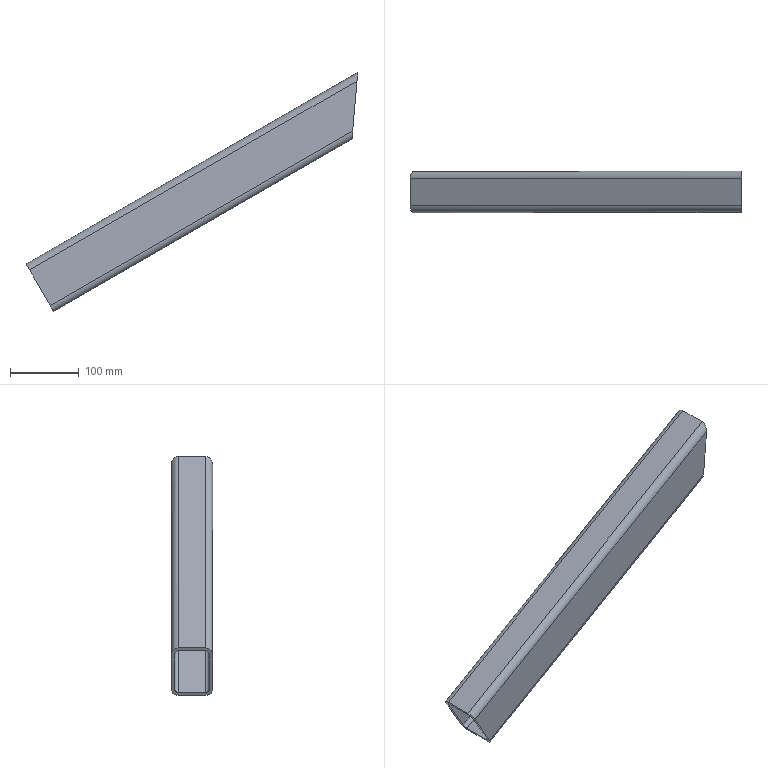Part | STEP file | front support column--000.001--20240925 | 1 solid | 18 faces | box 483.278 x 60 x 348.303 mm | volume 654919 mm3 | plane 10 | cylinder 8 | commonest cylinder face diameters 10 x4 20 x4